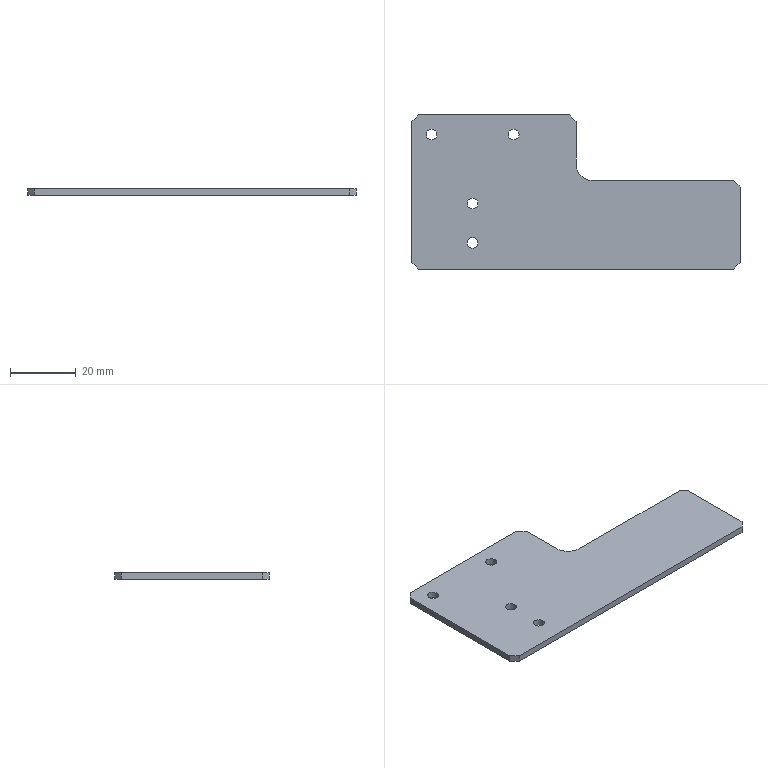Part | NX | 1 solid | 18 faces | box 100 x 47 x 2 mm | volume 7322 mm3 | plane 13 | cylinder 5 | commonest cylinder face diameters 3.3 x4 10 x1
STEP:
#1=CARTESIAN_POINT('',(-2.,23.5,0.));
#2=VERTEX_POINT('',#1);
#3=CARTESIAN_POINT('',(-48.,23.5,0.));
#4=VERTEX_POINT('',#3);
#5=CARTESIAN_POINT('',(50.,23.5,0.));
#6=DIRECTION('',(-1.,0.,0.));
#7=VECTOR('',#6,1000.);
#8=LINE('',#5,#7);
#9=EDGE_CURVE('',#2,#4,#8,.T.);
#10=ORIENTED_EDGE('',*,*,#9,.F.);
#11=CARTESIAN_POINT('',(-2.,23.5,-2.));
#12=VERTEX_POINT('',#11);
#13=CARTESIAN_POINT('',(-2.,23.5,-2.));
#14=DIRECTION('',(0.,0.,-1.));
#15=VECTOR('',#14,1000.);
#16=LINE('',#13,#15);
#17=EDGE_CURVE('',#2,#12,#16,.T.);
#18=ORIENTED_EDGE('',*,*,#17,.T.);
#19=CARTESIAN_POINT('',(-48.,23.5,-2.));
#20=VERTEX_POINT('',#19);
#21=CARTESIAN_POINT('',(50.,23.5,-2.));
#22=DIRECTION('',(-1.,0.,0.));
#23=VECTOR('',#22,1000.);
#24=LINE('',#21,#23);
#25=EDGE_CURVE('',#12,#20,#24,.T.);
#26=ORIENTED_EDGE('',*,*,#25,.T.);
#27=CARTESIAN_POINT('',(-48.,23.5,-2.));
#28=DIRECTION('',(0.,0.,1.));
#29=VECTOR('',#28,1000.);
#30=LINE('',#27,#29);
#31=EDGE_CURVE('',#20,#4,#30,.T.);
#32=ORIENTED_EDGE('',*,*,#31,.T.);
#33=EDGE_LOOP('',(#10,#18,#26,#32));
#34=FACE_BOUND('',#33,.T.);
#35=CARTESIAN_POINT('',(50.,23.5,-2.));
#36=DIRECTION('',(0.,1.,0.));
#37=DIRECTION('',(-1.,0.,0.));
#38=AXIS2_PLACEMENT_3D('',#35,#36,#37);
#39=PLANE('',#38);
#40=ADVANCED_FACE('',(#34),#39,.T.);
#41=CARTESIAN_POINT('',(50.,-21.5,-2.));
#42=VERTEX_POINT('',#41);
#43=CARTESIAN_POINT('',(50.,1.5,-2.));
#44=VERTEX_POINT('',#43);
#45=CARTESIAN_POINT('',(50.,-23.5,-2.));
#46=DIRECTION('',(0.,1.,0.));
#47=VECTOR('',#46,1000.);
#48=LINE('',#45,#47);
#49=EDGE_CURVE('',#42,#44,#48,.T.);
#50=ORIENTED_EDGE('',*,*,#49,.T.);
#51=CARTESIAN_POINT('',(50.,1.5,0.));
#52=VERTEX_POINT('',#51);
#53=CARTESIAN_POINT('',(50.,1.5,0.));
#54=DIRECTION('',(0.,0.,1.));
#55=VECTOR('',#54,1000.);
#56=LINE('',#53,#55);
#57=EDGE_CURVE('',#44,#52,#56,.T.);
#58=ORIENTED_EDGE('',*,*,#57,.T.);
#59=CARTESIAN_POINT('',(50.,-21.5,0.));
#60=VERTEX_POINT('',#59);
#61=CARTESIAN_POINT('',(50.,-23.5,0.));
#62=DIRECTION('',(0.,1.,0.));
#63=VECTOR('',#62,1000.);
#64=LINE('',#61,#63);
#65=EDGE_CURVE('',#60,#52,#64,.T.);
#66=ORIENTED_EDGE('',*,*,#65,.F.);
#67=CARTESIAN_POINT('',(50.,-21.5,-2.));
#68=DIRECTION('',(0.,0.,-1.));
#69=VECTOR('',#68,1000.);
#70=LINE('',#67,#69);
#71=EDGE_CURVE('',#60,#42,#70,.T.);
#72=ORIENTED_EDGE('',*,*,#71,.T.);
#73=EDGE_LOOP('',(#50,#58,#66,#72));
#74=FACE_BOUND('',#73,.T.);
#75=CARTESIAN_POINT('',(50.,-23.5,-2.));
#76=DIRECTION('',(1.,0.,0.));
#77=DIRECTION('',(0.,0.,-1.));
#78=AXIS2_PLACEMENT_3D('',#75,#76,#77);
#79=PLANE('',#78);
#80=ADVANCED_FACE('',(#74),#79,.T.);
#81=CARTESIAN_POINT('',(-48.,-23.5,0.));
#82=VERTEX_POINT('',#81);
#83=CARTESIAN_POINT('',(48.,-23.5,0.));
#84=VERTEX_POINT('',#83);
#85=CARTESIAN_POINT('',(-50.,-23.5,0.));
#86=DIRECTION('',(1.,0.,0.));
#87=VECTOR('',#86,1000.);
#88=LINE('',#85,#87);
#89=EDGE_CURVE('',#82,#84,#88,.T.);
#90=ORIENTED_EDGE('',*,*,#89,.F.);
#91=CARTESIAN_POINT('',(-48.,-23.5,-2.));
#92=VERTEX_POINT('',#91);
#93=CARTESIAN_POINT('',(-48.,-23.5,-2.));
#94=DIRECTION('',(0.,0.,-1.));
#95=VECTOR('',#94,1000.);
#96=LINE('',#93,#95);
#97=EDGE_CURVE('',#82,#92,#96,.T.);
#98=ORIENTED_EDGE('',*,*,#97,.T.);
#99=CARTESIAN_POINT('',(48.,-23.5,-2.));
#100=VERTEX_POINT('',#99);
#101=CARTESIAN_POINT('',(-50.,-23.5,-2.));
#102=DIRECTION('',(1.,0.,0.));
#103=VECTOR('',#102,1000.);
#104=LINE('',#101,#103);
#105=EDGE_CURVE('',#92,#100,#104,.T.);
#106=ORIENTED_EDGE('',*,*,#105,.T.);
#107=CARTESIAN_POINT('',(48.,-23.5,-2.));
#108=DIRECTION('',(0.,0.,1.));
#109=VECTOR('',#108,1000.);
#110=LINE('',#107,#109);
#111=EDGE_CURVE('',#100,#84,#110,.T.);
#112=ORIENTED_EDGE('',*,*,#111,.T.);
#113=EDGE_LOOP('',(#90,#98,#106,#112));
#114=FACE_BOUND('',#113,.T.);
#115=CARTESIAN_POINT('',(-50.,-23.5,-2.));
#116=DIRECTION('',(0.,-1.,0.));
#117=DIRECTION('',(0.,0.,-1.));
#118=AXIS2_PLACEMENT_3D('',#115,#116,#117);
#119=PLANE('',#118);
#120=ADVANCED_FACE('',(#114),#119,.T.);
#121=CARTESIAN_POINT('',(-50.,21.5,-2.));
#122=VERTEX_POINT('',#121);
#123=CARTESIAN_POINT('',(-50.,-21.5,-2.));
#124=VERTEX_POINT('',#123);
#125=CARTESIAN_POINT('',(-50.,23.5,-2.));
#126=DIRECTION('',(0.,-1.,0.));
#127=VECTOR('',#126,1000.);
#128=LINE('',#125,#127);
#129=EDGE_CURVE('',#122,#124,#128,.T.);
#130=ORIENTED_EDGE('',*,*,#129,.T.);
#131=CARTESIAN_POINT('',(-50.,-21.5,0.));
#132=VERTEX_POINT('',#131);
#133=CARTESIAN_POINT('',(-50.,-21.5,-2.));
#134=DIRECTION('',(0.,0.,1.));
#135=VECTOR('',#134,1000.);
#136=LINE('',#133,#135);
#137=EDGE_CURVE('',#124,#132,#136,.T.);
#138=ORIENTED_EDGE('',*,*,#137,.T.);
#139=CARTESIAN_POINT('',(-50.,21.5,0.));
#140=VERTEX_POINT('',#139);
#141=CARTESIAN_POINT('',(-50.,23.5,0.));
#142=DIRECTION('',(0.,-1.,0.));
#143=VECTOR('',#142,1000.);
#144=LINE('',#141,#143);
#145=EDGE_CURVE('',#140,#132,#144,.T.);
#146=ORIENTED_EDGE('',*,*,#145,.F.);
#147=CARTESIAN_POINT('',(-50.,21.5,-2.));
#148=DIRECTION('',(0.,0.,-1.));
#149=VECTOR('',#148,1000.);
#150=LINE('',#147,#149);
#151=EDGE_CURVE('',#140,#122,#150,.T.);
#152=ORIENTED_EDGE('',*,*,#151,.T.);
#153=EDGE_LOOP('',(#130,#138,#146,#152));
#154=FACE_BOUND('',#153,.T.);
#155=CARTESIAN_POINT('',(-50.,23.5,-2.));
#156=DIRECTION('',(-1.,0.,0.));
#157=DIRECTION('',(0.,0.,1.));
#158=AXIS2_PLACEMENT_3D('',#155,#156,#157);
#159=PLANE('',#158);
#160=ADVANCED_FACE('',(#154),#159,.T.);
#161=CARTESIAN_POINT('',(-29.85,-3.5,-2.));
#162=VERTEX_POINT('',#161);
#163=CARTESIAN_POINT('',(-31.5,-3.5,-2.));
#164=DIRECTION('',(0.,0.,1.));
#165=DIRECTION('',(1.,0.,0.));
#166=AXIS2_PLACEMENT_3D('',#163,#164,#165);
#167=CIRCLE('',#166,1.65);
#168=EDGE_CURVE('',#162,#162,#167,.T.);
#169=ORIENTED_EDGE('',*,*,#168,.T.);
#170=EDGE_LOOP('',(#169));
#171=FACE_BOUND('',#170,.T.);
#172=CARTESIAN_POINT('',(-29.85,-15.5,-2.));
#173=VERTEX_POINT('',#172);
#174=CARTESIAN_POINT('',(-31.5,-15.5,-2.));
#175=DIRECTION('',(0.,0.,1.));
#176=DIRECTION('',(1.,0.,0.));
#177=AXIS2_PLACEMENT_3D('',#174,#175,#176);
#178=CIRCLE('',#177,1.65);
#179=EDGE_CURVE('',#173,#173,#178,.T.);
#180=ORIENTED_EDGE('',*,*,#179,.T.);
#181=EDGE_LOOP('',(#180));
#182=FACE_BOUND('',#181,.T.);
#183=CARTESIAN_POINT('',(-42.35,17.5,-2.));
#184=VERTEX_POINT('',#183);
#185=CARTESIAN_POINT('',(-44.,17.5,-2.));
#186=DIRECTION('',(0.,0.,1.));
#187=DIRECTION('',(1.,0.,0.));
#188=AXIS2_PLACEMENT_3D('',#185,#186,#187);
#189=CIRCLE('',#188,1.65);
#190=EDGE_CURVE('',#184,#184,#189,.T.);
#191=ORIENTED_EDGE('',*,*,#190,.T.);
#192=EDGE_LOOP('',(#191));
#193=FACE_BOUND('',#192,.T.);
#194=CARTESIAN_POINT('',(-17.35,17.5,-2.));
#195=VERTEX_POINT('',#194);
#196=CARTESIAN_POINT('',(-19.,17.5,-2.));
#197=DIRECTION('',(0.,0.,1.));
#198=DIRECTION('',(1.,0.,0.));
#199=AXIS2_PLACEMENT_3D('',#196,#197,#198);
#200=CIRCLE('',#199,1.65);
#201=EDGE_CURVE('',#195,#195,#200,.T.);
#202=ORIENTED_EDGE('',*,*,#201,.T.);
#203=EDGE_LOOP('',(#202));
#204=FACE_BOUND('',#203,.T.);
#205=CARTESIAN_POINT('',(0.,21.5,-2.));
#206=VERTEX_POINT('',#205);
#207=CARTESIAN_POINT('',(0.,8.5,-2.));
#208=VERTEX_POINT('',#207);
#209=CARTESIAN_POINT('',(0.,23.5,-2.));
#210=DIRECTION('',(0.,-1.,0.));
#211=VECTOR('',#210,1000.);
#212=LINE('',#209,#211);
#213=EDGE_CURVE('',#206,#208,#212,.T.);
#214=ORIENTED_EDGE('',*,*,#213,.T.);
#215=CARTESIAN_POINT('',(5.,3.5,-2.));
#216=VERTEX_POINT('',#215);
#217=CARTESIAN_POINT('',(5.,8.5,-2.));
#218=DIRECTION('',(0.,0.,1.));
#219=DIRECTION('',(1.,0.,0.));
#220=AXIS2_PLACEMENT_3D('',#217,#218,#219);
#221=CIRCLE('',#220,5.);
#222=EDGE_CURVE('',#208,#216,#221,.T.);
#223=ORIENTED_EDGE('',*,*,#222,.T.);
#224=CARTESIAN_POINT('',(48.,3.5,-2.));
#225=VERTEX_POINT('',#224);
#226=CARTESIAN_POINT('',(50.,3.5,-2.));
#227=DIRECTION('',(1.,0.,0.));
#228=VECTOR('',#227,1000.);
#229=LINE('',#226,#228);
#230=EDGE_CURVE('',#216,#225,#229,.T.);
#231=ORIENTED_EDGE('',*,*,#230,.T.);
#232=CARTESIAN_POINT('',(50.,1.5,-2.));
#233=DIRECTION('',(0.7071,-0.7071,0.));
#234=VECTOR('',#233,1000.);
#235=LINE('',#232,#234);
#236=EDGE_CURVE('',#225,#44,#235,.T.);
#237=ORIENTED_EDGE('',*,*,#236,.T.);
#238=ORIENTED_EDGE('',*,*,#49,.F.);
#239=CARTESIAN_POINT('',(48.,-23.5,-2.));
#240=DIRECTION('',(0.7071,0.7071,0.));
#241=VECTOR('',#240,1000.);
#242=LINE('',#239,#241);
#243=EDGE_CURVE('',#42,#100,#242,.F.);
#244=ORIENTED_EDGE('',*,*,#243,.T.);
#245=ORIENTED_EDGE('',*,*,#105,.F.);
#246=CARTESIAN_POINT('',(-50.,-21.5,-2.));
#247=DIRECTION('',(0.7071,-0.7071,0.));
#248=VECTOR('',#247,1000.);
#249=LINE('',#246,#248);
#250=EDGE_CURVE('',#92,#124,#249,.F.);
#251=ORIENTED_EDGE('',*,*,#250,.T.);
#252=ORIENTED_EDGE('',*,*,#129,.F.);
#253=CARTESIAN_POINT('',(-48.,23.5,-2.));
#254=DIRECTION('',(-0.7071,-0.7071,0.));
#255=VECTOR('',#254,1000.);
#256=LINE('',#253,#255);
#257=EDGE_CURVE('',#122,#20,#256,.F.);
#258=ORIENTED_EDGE('',*,*,#257,.T.);
#259=ORIENTED_EDGE('',*,*,#25,.F.);
#260=CARTESIAN_POINT('',(0.,21.5,-2.));
#261=DIRECTION('',(0.7071,-0.7071,0.));
#262=VECTOR('',#261,1000.);
#263=LINE('',#260,#262);
#264=EDGE_CURVE('',#12,#206,#263,.T.);
#265=ORIENTED_EDGE('',*,*,#264,.T.);
#266=EDGE_LOOP('',(#214,#223,#231,#237,#238,#244,#245,#251,#252,#258,#259,#265));
#267=FACE_BOUND('',#266,.T.);
#268=CARTESIAN_POINT('',(0.,0.,-2.));
#269=DIRECTION('',(0.,0.,1.));
#270=DIRECTION('',(1.,0.,0.));
#271=AXIS2_PLACEMENT_3D('',#268,#269,#270);
#272=PLANE('',#271);
#273=ADVANCED_FACE('',(#171,#182,#193,#204,#267),#272,.F.);
#274=ORIENTED_EDGE('',*,*,#65,.T.);
#275=CARTESIAN_POINT('',(48.,3.5,0.));
#276=VERTEX_POINT('',#275);
#277=CARTESIAN_POINT('',(25.75,25.75,0.));
#278=DIRECTION('',(-0.7071,0.7071,0.));
#279=VECTOR('',#278,1000.);
#280=LINE('',#277,#279);
#281=EDGE_CURVE('',#52,#276,#280,.T.);
#282=ORIENTED_EDGE('',*,*,#281,.T.);
#283=CARTESIAN_POINT('',(5.,3.5,0.));
#284=VERTEX_POINT('',#283);
#285=CARTESIAN_POINT('',(50.,3.5,0.));
#286=DIRECTION('',(1.,0.,0.));
#287=VECTOR('',#286,1000.);
#288=LINE('',#285,#287);
#289=EDGE_CURVE('',#284,#276,#288,.T.);
#290=ORIENTED_EDGE('',*,*,#289,.F.);
#291=CARTESIAN_POINT('',(0.,8.5,0.));
#292=VERTEX_POINT('',#291);
#293=CARTESIAN_POINT('',(5.,8.5,0.));
#294=DIRECTION('',(0.,0.,1.));
#295=DIRECTION('',(1.,0.,0.));
#296=AXIS2_PLACEMENT_3D('',#293,#294,#295);
#297=CIRCLE('',#296,5.);
#298=EDGE_CURVE('',#284,#292,#297,.F.);
#299=ORIENTED_EDGE('',*,*,#298,.T.);
#300=CARTESIAN_POINT('',(0.,21.5,0.));
#301=VERTEX_POINT('',#300);
#302=CARTESIAN_POINT('',(0.,23.5,0.));
#303=DIRECTION('',(0.,-1.,0.));
#304=VECTOR('',#303,1000.);
#305=LINE('',#302,#304);
#306=EDGE_CURVE('',#301,#292,#305,.T.);
#307=ORIENTED_EDGE('',*,*,#306,.F.);
#308=CARTESIAN_POINT('',(10.75,10.75,0.));
#309=DIRECTION('',(-0.7071,0.7071,0.));
#310=VECTOR('',#309,1000.);
#311=LINE('',#308,#310);
#312=EDGE_CURVE('',#301,#2,#311,.T.);
#313=ORIENTED_EDGE('',*,*,#312,.T.);
#314=ORIENTED_EDGE('',*,*,#9,.T.);
#315=CARTESIAN_POINT('',(-35.75,35.75,0.));
#316=DIRECTION('',(0.7071,0.7071,0.));
#317=VECTOR('',#316,1000.);
#318=LINE('',#315,#317);
#319=EDGE_CURVE('',#4,#140,#318,.F.);
#320=ORIENTED_EDGE('',*,*,#319,.T.);
#321=ORIENTED_EDGE('',*,*,#145,.T.);
#322=CARTESIAN_POINT('',(-35.75,-35.75,0.));
#323=DIRECTION('',(-0.7071,0.7071,0.));
#324=VECTOR('',#323,1000.);
#325=LINE('',#322,#324);
#326=EDGE_CURVE('',#132,#82,#325,.F.);
#327=ORIENTED_EDGE('',*,*,#326,.T.);
#328=ORIENTED_EDGE('',*,*,#89,.T.);
#329=CARTESIAN_POINT('',(35.75,-35.75,0.));
#330=DIRECTION('',(-0.7071,-0.7071,0.));
#331=VECTOR('',#330,1000.);
#332=LINE('',#329,#331);
#333=EDGE_CURVE('',#84,#60,#332,.F.);
#334=ORIENTED_EDGE('',*,*,#333,.T.);
#335=EDGE_LOOP('',(#274,#282,#290,#299,#307,#313,#314,#320,#321,#327,#328,#334));
#336=FACE_BOUND('',#335,.T.);
#337=CARTESIAN_POINT('',(-29.85,-3.5,0.));
#338=VERTEX_POINT('',#337);
#339=CARTESIAN_POINT('',(-31.5,-3.5,0.));
#340=DIRECTION('',(0.,0.,1.));
#341=DIRECTION('',(1.,0.,0.));
#342=AXIS2_PLACEMENT_3D('',#339,#340,#341);
#343=CIRCLE('',#342,1.65);
#344=EDGE_CURVE('',#338,#338,#343,.T.);
#345=ORIENTED_EDGE('',*,*,#344,.F.);
#346=EDGE_LOOP('',(#345));
#347=FACE_BOUND('',#346,.T.);
#348=CARTESIAN_POINT('',(-29.85,-15.5,0.));
#349=VERTEX_POINT('',#348);
#350=CARTESIAN_POINT('',(-31.5,-15.5,0.));
#351=DIRECTION('',(0.,0.,1.));
#352=DIRECTION('',(1.,0.,0.));
#353=AXIS2_PLACEMENT_3D('',#350,#351,#352);
#354=CIRCLE('',#353,1.65);
#355=EDGE_CURVE('',#349,#349,#354,.T.);
#356=ORIENTED_EDGE('',*,*,#355,.F.);
#357=EDGE_LOOP('',(#356));
#358=FACE_BOUND('',#357,.T.);
#359=CARTESIAN_POINT('',(-42.35,17.5,0.));
#360=VERTEX_POINT('',#359);
#361=CARTESIAN_POINT('',(-44.,17.5,0.));
#362=DIRECTION('',(0.,0.,1.));
#363=DIRECTION('',(1.,0.,0.));
#364=AXIS2_PLACEMENT_3D('',#361,#362,#363);
#365=CIRCLE('',#364,1.65);
#366=EDGE_CURVE('',#360,#360,#365,.T.);
#367=ORIENTED_EDGE('',*,*,#366,.F.);
#368=EDGE_LOOP('',(#367));
#369=FACE_BOUND('',#368,.T.);
#370=CARTESIAN_POINT('',(-17.35,17.5,0.));
#371=VERTEX_POINT('',#370);
#372=CARTESIAN_POINT('',(-19.,17.5,0.));
#373=DIRECTION('',(0.,0.,1.));
#374=DIRECTION('',(1.,0.,0.));
#375=AXIS2_PLACEMENT_3D('',#372,#373,#374);
#376=CIRCLE('',#375,1.65);
#377=EDGE_CURVE('',#371,#371,#376,.T.);
#378=ORIENTED_EDGE('',*,*,#377,.F.);
#379=EDGE_LOOP('',(#378));
#380=FACE_BOUND('',#379,.T.);
#381=CARTESIAN_POINT('',(0.,0.,0.));
#382=DIRECTION('',(0.,0.,1.));
#383=DIRECTION('',(1.,0.,0.));
#384=AXIS2_PLACEMENT_3D('',#381,#382,#383);
#385=PLANE('',#384);
#386=ADVANCED_FACE('',(#336,#347,#358,#369,#380),#385,.T.);
#387=ORIENTED_EDGE('',*,*,#201,.F.);
#388=EDGE_LOOP('',(#387));
#389=FACE_BOUND('',#388,.T.);
#390=ORIENTED_EDGE('',*,*,#377,.T.);
#391=EDGE_LOOP('',(#390));
#392=FACE_BOUND('',#391,.T.);
#393=CARTESIAN_POINT('',(-19.,17.5,0.));
#394=DIRECTION('',(0.,0.,1.));
#395=DIRECTION('',(1.,0.,0.));
#396=AXIS2_PLACEMENT_3D('',#393,#394,#395);
#397=CYLINDRICAL_SURFACE('',#396,1.65);
#398=ADVANCED_FACE('',(#389,#392),#397,.F.);
#399=ORIENTED_EDGE('',*,*,#190,.F.);
#400=EDGE_LOOP('',(#399));
#401=FACE_BOUND('',#400,.T.);
#402=ORIENTED_EDGE('',*,*,#366,.T.);
#403=EDGE_LOOP('',(#402));
#404=FACE_BOUND('',#403,.T.);
#405=CARTESIAN_POINT('',(-44.,17.5,0.));
#406=DIRECTION('',(0.,0.,1.));
#407=DIRECTION('',(1.,0.,0.));
#408=AXIS2_PLACEMENT_3D('',#405,#406,#407);
#409=CYLINDRICAL_SURFACE('',#408,1.65);
#410=ADVANCED_FACE('',(#401,#404),#409,.F.);
#411=ORIENTED_EDGE('',*,*,#179,.F.);
#412=EDGE_LOOP('',(#411));
#413=FACE_BOUND('',#412,.T.);
#414=ORIENTED_EDGE('',*,*,#355,.T.);
#415=EDGE_LOOP('',(#414));
#416=FACE_BOUND('',#415,.T.);
#417=CARTESIAN_POINT('',(-31.5,-15.5,0.));
#418=DIRECTION('',(0.,0.,1.));
#419=DIRECTION('',(1.,0.,0.));
#420=AXIS2_PLACEMENT_3D('',#417,#418,#419);
#421=CYLINDRICAL_SURFACE('',#420,1.65);
#422=ADVANCED_FACE('',(#413,#416),#421,.F.);
#423=ORIENTED_EDGE('',*,*,#168,.F.);
#424=EDGE_LOOP('',(#423));
#425=FACE_BOUND('',#424,.T.);
#426=ORIENTED_EDGE('',*,*,#344,.T.);
#427=EDGE_LOOP('',(#426));
#428=FACE_BOUND('',#427,.T.);
#429=CARTESIAN_POINT('',(-31.5,-3.5,0.));
#430=DIRECTION('',(0.,0.,1.));
#431=DIRECTION('',(1.,0.,0.));
#432=AXIS2_PLACEMENT_3D('',#429,#430,#431);
#433=CYLINDRICAL_SURFACE('',#432,1.65);
#434=ADVANCED_FACE('',(#425,#428),#433,.F.);
#435=ORIENTED_EDGE('',*,*,#230,.F.);
#436=CARTESIAN_POINT('',(5.,3.5,0.));
#437=DIRECTION('',(0.,0.,1.));
#438=VECTOR('',#437,1000.);
#439=LINE('',#436,#438);
#440=EDGE_CURVE('',#216,#284,#439,.T.);
#441=ORIENTED_EDGE('',*,*,#440,.T.);
#442=ORIENTED_EDGE('',*,*,#289,.T.);
#443=CARTESIAN_POINT('',(48.,3.5,-2.));
#444=DIRECTION('',(0.,0.,-1.));
#445=VECTOR('',#444,1000.);
#446=LINE('',#443,#445);
#447=EDGE_CURVE('',#276,#225,#446,.T.);
#448=ORIENTED_EDGE('',*,*,#447,.T.);
#449=EDGE_LOOP('',(#435,#441,#442,#448));
#450=FACE_BOUND('',#449,.T.);
#451=CARTESIAN_POINT('',(50.,3.5,-2.));
#452=DIRECTION('',(0.,-1.,0.));
#453=DIRECTION('',(1.,0.,0.));
#454=AXIS2_PLACEMENT_3D('',#451,#452,#453);
#455=PLANE('',#454);
#456=ADVANCED_FACE('',(#450),#455,.F.);
#457=ORIENTED_EDGE('',*,*,#306,.T.);
#458=CARTESIAN_POINT('',(0.,8.5,-2.));
#459=DIRECTION('',(0.,0.,1.));
#460=VECTOR('',#459,1000.);
#461=LINE('',#458,#460);
#462=EDGE_CURVE('',#292,#208,#461,.F.);
#463=ORIENTED_EDGE('',*,*,#462,.T.);
#464=ORIENTED_EDGE('',*,*,#213,.F.);
#465=CARTESIAN_POINT('',(0.,21.5,0.));
#466=DIRECTION('',(0.,0.,1.));
#467=VECTOR('',#466,1000.);
#468=LINE('',#465,#467);
#469=EDGE_CURVE('',#206,#301,#468,.T.);
#470=ORIENTED_EDGE('',*,*,#469,.T.);
#471=EDGE_LOOP('',(#457,#463,#464,#470));
#472=FACE_BOUND('',#471,.T.);
#473=CARTESIAN_POINT('',(0.,23.5,-2.));
#474=DIRECTION('',(-1.,0.,0.));
#475=DIRECTION('',(0.,0.,1.));
#476=AXIS2_PLACEMENT_3D('',#473,#474,#475);
#477=PLANE('',#476);
#478=ADVANCED_FACE('',(#472),#477,.F.);
#479=ORIENTED_EDGE('',*,*,#236,.F.);
#480=ORIENTED_EDGE('',*,*,#447,.F.);
#481=ORIENTED_EDGE('',*,*,#281,.F.);
#482=ORIENTED_EDGE('',*,*,#57,.F.);
#483=EDGE_LOOP('',(#479,#480,#481,#482));
#484=FACE_BOUND('',#483,.T.);
#485=CARTESIAN_POINT('',(50.,1.5,-2.));
#486=DIRECTION('',(0.7071,0.7071,0.));
#487=DIRECTION('',(0.,0.,-1.));
#488=AXIS2_PLACEMENT_3D('',#485,#486,#487);
#489=PLANE('',#488);
#490=ADVANCED_FACE('',(#484),#489,.T.);
#491=ORIENTED_EDGE('',*,*,#264,.F.);
#492=ORIENTED_EDGE('',*,*,#17,.F.);
#493=ORIENTED_EDGE('',*,*,#312,.F.);
#494=ORIENTED_EDGE('',*,*,#469,.F.);
#495=EDGE_LOOP('',(#491,#492,#493,#494));
#496=FACE_BOUND('',#495,.T.);
#497=CARTESIAN_POINT('',(0.,21.5,-2.));
#498=DIRECTION('',(0.7071,0.7071,0.));
#499=DIRECTION('',(0.,0.,-1.));
#500=AXIS2_PLACEMENT_3D('',#497,#498,#499);
#501=PLANE('',#500);
#502=ADVANCED_FACE('',(#496),#501,.T.);
#503=ORIENTED_EDGE('',*,*,#250,.F.);
#504=ORIENTED_EDGE('',*,*,#97,.F.);
#505=ORIENTED_EDGE('',*,*,#326,.F.);
#506=ORIENTED_EDGE('',*,*,#137,.F.);
#507=EDGE_LOOP('',(#503,#504,#505,#506));
#508=FACE_BOUND('',#507,.T.);
#509=CARTESIAN_POINT('',(-50.,-21.5,-2.));
#510=DIRECTION('',(0.7071,0.7071,0.));
#511=DIRECTION('',(0.,0.,1.));
#512=AXIS2_PLACEMENT_3D('',#509,#510,#511);
#513=PLANE('',#512);
#514=ADVANCED_FACE('',(#508),#513,.F.);
#515=ORIENTED_EDGE('',*,*,#257,.F.);
#516=ORIENTED_EDGE('',*,*,#151,.F.);
#517=ORIENTED_EDGE('',*,*,#319,.F.);
#518=ORIENTED_EDGE('',*,*,#31,.F.);
#519=EDGE_LOOP('',(#515,#516,#517,#518));
#520=FACE_BOUND('',#519,.T.);
#521=CARTESIAN_POINT('',(-48.,23.5,-2.));
#522=DIRECTION('',(0.7071,-0.7071,0.));
#523=DIRECTION('',(0.,0.,1.));
#524=AXIS2_PLACEMENT_3D('',#521,#522,#523);
#525=PLANE('',#524);
#526=ADVANCED_FACE('',(#520),#525,.F.);
#527=ORIENTED_EDGE('',*,*,#243,.F.);
#528=ORIENTED_EDGE('',*,*,#71,.F.);
#529=ORIENTED_EDGE('',*,*,#333,.F.);
#530=ORIENTED_EDGE('',*,*,#111,.F.);
#531=EDGE_LOOP('',(#527,#528,#529,#530));
#532=FACE_BOUND('',#531,.T.);
#533=CARTESIAN_POINT('',(48.,-23.5,-2.));
#534=DIRECTION('',(-0.7071,0.7071,0.));
#535=DIRECTION('',(0.,0.,1.));
#536=AXIS2_PLACEMENT_3D('',#533,#534,#535);
#537=PLANE('',#536);
#538=ADVANCED_FACE('',(#532),#537,.F.);
#539=ORIENTED_EDGE('',*,*,#222,.F.);
#540=ORIENTED_EDGE('',*,*,#462,.F.);
#541=ORIENTED_EDGE('',*,*,#298,.F.);
#542=ORIENTED_EDGE('',*,*,#440,.F.);
#543=EDGE_LOOP('',(#539,#540,#541,#542));
#544=FACE_BOUND('',#543,.T.);
#545=CARTESIAN_POINT('',(5.,8.5,-2.));
#546=DIRECTION('',(0.,0.,-1.));
#547=DIRECTION('',(-1.,0.,0.));
#548=AXIS2_PLACEMENT_3D('',#545,#546,#547);
#549=CYLINDRICAL_SURFACE('',#548,5.);
#550=ADVANCED_FACE('',(#544),#549,.F.);
#551=CLOSED_SHELL('',(#40,#80,#120,#160,#273,#386,#398,#410,#422,#434,#456,#478,#490,#502,#514,#526,#538,#550));
#552=MANIFOLD_SOLID_BREP('',#551);
#553=(LENGTH_UNIT()NAMED_UNIT(*)SI_UNIT(.MILLI.,.METRE.));
#554=UNCERTAINTY_MEASURE_WITH_UNIT(LENGTH_MEASURE(0.00001),#553,'','');
#555=(NAMED_UNIT(*)PLANE_ANGLE_UNIT()SI_UNIT($,.RADIAN.));
#556=(NAMED_UNIT(*)SI_UNIT($,.STERADIAN.)SOLID_ANGLE_UNIT());
#557=(GEOMETRIC_REPRESENTATION_CONTEXT(3)GLOBAL_UNCERTAINTY_ASSIGNED_CONTEXT((#554))GLOBAL_UNIT_ASSIGNED_CONTEXT((#553,#555,#556))REPRESENTATION_CONTEXT('',''));
#558=ADVANCED_BREP_SHAPE_REPRESENTATION('',(#552),#557);